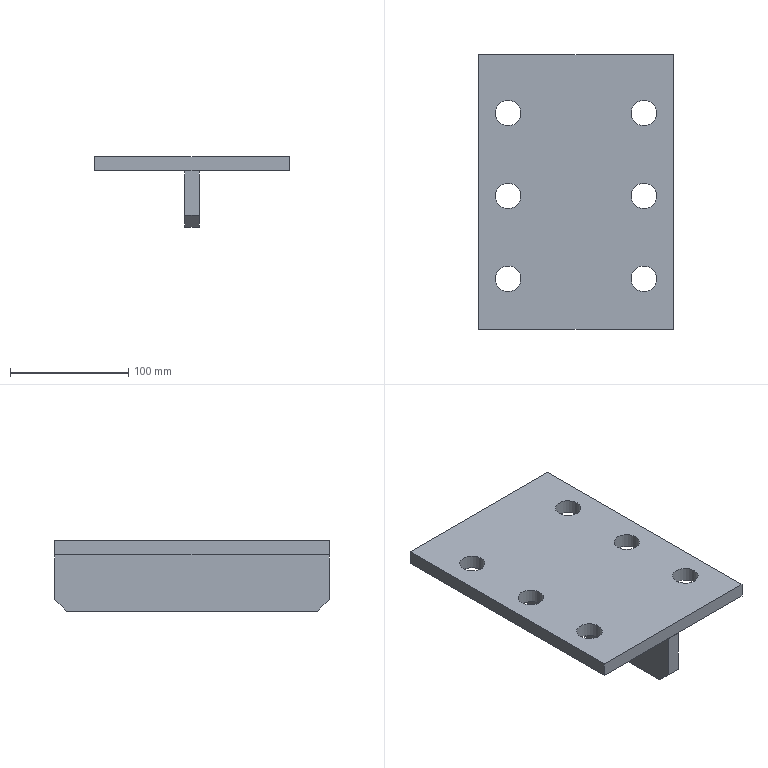Part | STEP file | PN_0033 beam connector 12t_Default<As Machined> | 2 solids | 20 faces | box 164.5 x 232 x 59.5 mm | volume 562868 mm3 | plane 14 | cylinder 6 | commonest cylinder face diameters 21.5 x6
STEP:
#1=CARTESIAN_POINT('',(0.,0.,0.));
#2=DIRECTION('',(0.,0.,1.));
#3=DIRECTION('',(1.,0.,0.));
#4=AXIS2_PLACEMENT_3D('',#1,#2,#3);
#5=CARTESIAN_POINT('',(-6.,-116.,-37.5));
#6=VERTEX_POINT('',#5);
#7=CARTESIAN_POINT('',(6.,-116.,-37.5));
#8=VERTEX_POINT('',#7);
#9=CARTESIAN_POINT('',(6.,-116.,-37.5));
#10=DIRECTION('',(1.,0.,0.));
#11=VECTOR('',#10,1.);
#12=LINE('',#9,#11);
#13=CARTESIAN_POINT('',(6.,-116.,-37.5));
#14=DIRECTION('',(0.,0.7071,0.7071));
#15=DIRECTION('',(1.,0.,0.));
#16=AXIS2_PLACEMENT_3D('',#13,#14,#15);
#17=PLANE('',#16);
#18=CARTESIAN_POINT('',(0.,0.));
#19=DIRECTION('',(1.,0.));
#20=VECTOR('',#19,1.);
#21=LINE('',#18,#20);
#22=(GEOMETRIC_REPRESENTATION_CONTEXT(2)PARAMETRIC_REPRESENTATION_CONTEXT()REPRESENTATION_CONTEXT('',''));
#23=DEFINITIONAL_REPRESENTATION('',(#21),#22);
#24=PCURVE('',#17,#23);
#25=CARTESIAN_POINT('',(6.,-116.,0.));
#26=DIRECTION('',(0.,1.,0.));
#27=DIRECTION('',(0.,0.,1.));
#28=AXIS2_PLACEMENT_3D('',#25,#26,#27);
#29=PLANE('',#28);
#30=CARTESIAN_POINT('',(-37.5,0.));
#31=DIRECTION('',(0.,1.));
#32=VECTOR('',#31,1.);
#33=LINE('',#30,#32);
#34=(GEOMETRIC_REPRESENTATION_CONTEXT(2)PARAMETRIC_REPRESENTATION_CONTEXT()REPRESENTATION_CONTEXT('',''));
#35=DEFINITIONAL_REPRESENTATION('',(#33),#34);
#36=PCURVE('',#29,#35);
#37=SURFACE_CURVE('',#12,(#24,#36),.PCURVE_S1.);
#38=EDGE_CURVE('',#6,#8,#37,.T.);
#39=ORIENTED_EDGE('',*,*,#38,.F.);
#40=CARTESIAN_POINT('',(-6.,-106.,-47.5));
#41=VERTEX_POINT('',#40);
#42=CARTESIAN_POINT('',(-6.,-116.,-37.5));
#43=DIRECTION('',(0.,-0.7071,0.7071));
#44=VECTOR('',#43,1.);
#45=LINE('',#42,#44);
#46=CARTESIAN_POINT('',(-12.,0.));
#47=DIRECTION('',(0.,-1.));
#48=VECTOR('',#47,1.);
#49=LINE('',#46,#48);
#50=(GEOMETRIC_REPRESENTATION_CONTEXT(2)PARAMETRIC_REPRESENTATION_CONTEXT()REPRESENTATION_CONTEXT('',''));
#51=DEFINITIONAL_REPRESENTATION('',(#49),#50);
#52=PCURVE('',#17,#51);
#53=CARTESIAN_POINT('',(-6.,0.,-23.75));
#54=DIRECTION('',(1.,0.,0.));
#55=DIRECTION('',(0.,0.,-1.));
#56=AXIS2_PLACEMENT_3D('',#53,#54,#55);
#57=PLANE('',#56);
#58=CARTESIAN_POINT('',(13.75,-116.));
#59=DIRECTION('',(-0.7071,-0.7071));
#60=VECTOR('',#59,1.);
#61=LINE('',#58,#60);
#62=(GEOMETRIC_REPRESENTATION_CONTEXT(2)PARAMETRIC_REPRESENTATION_CONTEXT()REPRESENTATION_CONTEXT('',''));
#63=DEFINITIONAL_REPRESENTATION('',(#61),#62);
#64=PCURVE('',#57,#63);
#65=SURFACE_CURVE('',#45,(#52,#64),.PCURVE_S1.);
#66=EDGE_CURVE('',#41,#6,#65,.T.);
#67=ORIENTED_EDGE('',*,*,#66,.F.);
#68=CARTESIAN_POINT('',(6.,-106.,-47.5));
#69=VERTEX_POINT('',#68);
#70=CARTESIAN_POINT('',(6.,-106.,-47.5));
#71=DIRECTION('',(-1.,0.,0.));
#72=VECTOR('',#71,1.);
#73=LINE('',#70,#72);
#74=CARTESIAN_POINT('',(0.,14.142));
#75=DIRECTION('',(-1.,0.));
#76=VECTOR('',#75,1.);
#77=LINE('',#74,#76);
#78=(GEOMETRIC_REPRESENTATION_CONTEXT(2)PARAMETRIC_REPRESENTATION_CONTEXT()REPRESENTATION_CONTEXT('',''));
#79=DEFINITIONAL_REPRESENTATION('',(#77),#78);
#80=PCURVE('',#17,#79);
#81=CARTESIAN_POINT('',(6.,116.,-47.5));
#82=DIRECTION('',(0.,0.,1.));
#83=DIRECTION('',(1.,0.,0.));
#84=AXIS2_PLACEMENT_3D('',#81,#82,#83);
#85=PLANE('',#84);
#86=CARTESIAN_POINT('',(0.,-222.));
#87=DIRECTION('',(-1.,0.));
#88=VECTOR('',#87,1.);
#89=LINE('',#86,#88);
#90=(GEOMETRIC_REPRESENTATION_CONTEXT(2)PARAMETRIC_REPRESENTATION_CONTEXT()REPRESENTATION_CONTEXT('',''));
#91=DEFINITIONAL_REPRESENTATION('',(#89),#90);
#92=PCURVE('',#85,#91);
#93=SURFACE_CURVE('',#73,(#80,#92),.PCURVE_S1.);
#94=EDGE_CURVE('',#69,#41,#93,.T.);
#95=ORIENTED_EDGE('',*,*,#94,.F.);
#96=CARTESIAN_POINT('',(6.,-64.875,-88.625));
#97=DIRECTION('',(0.,0.7071,-0.7071));
#98=VECTOR('',#97,1.);
#99=LINE('',#96,#98);
#100=CARTESIAN_POINT('',(0.,72.302));
#101=DIRECTION('',(0.,1.));
#102=VECTOR('',#101,1.);
#103=LINE('',#100,#102);
#104=(GEOMETRIC_REPRESENTATION_CONTEXT(2)PARAMETRIC_REPRESENTATION_CONTEXT()REPRESENTATION_CONTEXT('',''));
#105=DEFINITIONAL_REPRESENTATION('',(#103),#104);
#106=PCURVE('',#17,#105);
#107=CARTESIAN_POINT('',(6.,0.,-23.75));
#108=DIRECTION('',(1.,0.,0.));
#109=DIRECTION('',(0.,0.,-1.));
#110=AXIS2_PLACEMENT_3D('',#107,#108,#109);
#111=PLANE('',#110);
#112=CARTESIAN_POINT('',(64.875,-64.875));
#113=DIRECTION('',(0.7071,0.7071));
#114=VECTOR('',#113,1.);
#115=LINE('',#112,#114);
#116=(GEOMETRIC_REPRESENTATION_CONTEXT(2)PARAMETRIC_REPRESENTATION_CONTEXT()REPRESENTATION_CONTEXT('',''));
#117=DEFINITIONAL_REPRESENTATION('',(#115),#116);
#118=PCURVE('',#111,#117);
#119=SURFACE_CURVE('',#99,(#106,#118),.PCURVE_S1.);
#120=EDGE_CURVE('',#8,#69,#119,.T.);
#121=ORIENTED_EDGE('',*,*,#120,.F.);
#122=EDGE_LOOP('',(#39,#67,#95,#121));
#123=FACE_BOUND('',#122,.T.);
#124=ADVANCED_FACE('',(#123),#17,.F.);
#125=CARTESIAN_POINT('',(6.,116.,-37.5));
#126=VERTEX_POINT('',#125);
#127=CARTESIAN_POINT('',(-6.,116.,-37.5));
#128=VERTEX_POINT('',#127);
#129=CARTESIAN_POINT('',(6.,116.,-37.5));
#130=DIRECTION('',(-1.,0.,0.));
#131=VECTOR('',#130,1.);
#132=LINE('',#129,#131);
#133=CARTESIAN_POINT('',(6.,116.,-37.5));
#134=DIRECTION('',(0.,-0.7071,0.7071));
#135=DIRECTION('',(-1.,0.,0.));
#136=AXIS2_PLACEMENT_3D('',#133,#134,#135);
#137=PLANE('',#136);
#138=CARTESIAN_POINT('',(0.,0.));
#139=DIRECTION('',(1.,0.));
#140=VECTOR('',#139,1.);
#141=LINE('',#138,#140);
#142=(GEOMETRIC_REPRESENTATION_CONTEXT(2)PARAMETRIC_REPRESENTATION_CONTEXT()REPRESENTATION_CONTEXT('',''));
#143=DEFINITIONAL_REPRESENTATION('',(#141),#142);
#144=PCURVE('',#137,#143);
#145=CARTESIAN_POINT('',(6.,116.,0.));
#146=DIRECTION('',(0.,-1.,0.));
#147=DIRECTION('',(0.,0.,-1.));
#148=AXIS2_PLACEMENT_3D('',#145,#146,#147);
#149=PLANE('',#148);
#150=CARTESIAN_POINT('',(37.5,0.));
#151=DIRECTION('',(0.,-1.));
#152=VECTOR('',#151,1.);
#153=LINE('',#150,#152);
#154=(GEOMETRIC_REPRESENTATION_CONTEXT(2)PARAMETRIC_REPRESENTATION_CONTEXT()REPRESENTATION_CONTEXT('',''));
#155=DEFINITIONAL_REPRESENTATION('',(#153),#154);
#156=PCURVE('',#149,#155);
#157=SURFACE_CURVE('',#132,(#144,#156),.PCURVE_S1.);
#158=EDGE_CURVE('',#126,#128,#157,.T.);
#159=ORIENTED_EDGE('',*,*,#158,.F.);
#160=CARTESIAN_POINT('',(6.,106.,-47.5));
#161=VERTEX_POINT('',#160);
#162=CARTESIAN_POINT('',(6.,64.875,-88.625));
#163=DIRECTION('',(0.,0.7071,0.7071));
#164=VECTOR('',#163,1.);
#165=LINE('',#162,#164);
#166=CARTESIAN_POINT('',(0.,72.302));
#167=DIRECTION('',(0.,-1.));
#168=VECTOR('',#167,1.);
#169=LINE('',#166,#168);
#170=(GEOMETRIC_REPRESENTATION_CONTEXT(2)PARAMETRIC_REPRESENTATION_CONTEXT()REPRESENTATION_CONTEXT('',''));
#171=DEFINITIONAL_REPRESENTATION('',(#169),#170);
#172=PCURVE('',#137,#171);
#173=CARTESIAN_POINT('',(64.875,64.875));
#174=DIRECTION('',(-0.7071,0.7071));
#175=VECTOR('',#174,1.);
#176=LINE('',#173,#175);
#177=(GEOMETRIC_REPRESENTATION_CONTEXT(2)PARAMETRIC_REPRESENTATION_CONTEXT()REPRESENTATION_CONTEXT('',''));
#178=DEFINITIONAL_REPRESENTATION('',(#176),#177);
#179=PCURVE('',#111,#178);
#180=SURFACE_CURVE('',#165,(#172,#179),.PCURVE_S1.);
#181=EDGE_CURVE('',#161,#126,#180,.T.);
#182=ORIENTED_EDGE('',*,*,#181,.F.);
#183=CARTESIAN_POINT('',(-6.,106.,-47.5));
#184=VERTEX_POINT('',#183);
#185=CARTESIAN_POINT('',(6.,106.,-47.5));
#186=DIRECTION('',(1.,0.,0.));
#187=VECTOR('',#186,1.);
#188=LINE('',#185,#187);
#189=CARTESIAN_POINT('',(0.,14.142));
#190=DIRECTION('',(-1.,0.));
#191=VECTOR('',#190,1.);
#192=LINE('',#189,#191);
#193=(GEOMETRIC_REPRESENTATION_CONTEXT(2)PARAMETRIC_REPRESENTATION_CONTEXT()REPRESENTATION_CONTEXT('',''));
#194=DEFINITIONAL_REPRESENTATION('',(#192),#193);
#195=PCURVE('',#137,#194);
#196=CARTESIAN_POINT('',(0.,-10.));
#197=DIRECTION('',(1.,0.));
#198=VECTOR('',#197,1.);
#199=LINE('',#196,#198);
#200=(GEOMETRIC_REPRESENTATION_CONTEXT(2)PARAMETRIC_REPRESENTATION_CONTEXT()REPRESENTATION_CONTEXT('',''));
#201=DEFINITIONAL_REPRESENTATION('',(#199),#200);
#202=PCURVE('',#85,#201);
#203=SURFACE_CURVE('',#188,(#195,#202),.PCURVE_S1.);
#204=EDGE_CURVE('',#184,#161,#203,.T.);
#205=ORIENTED_EDGE('',*,*,#204,.F.);
#206=CARTESIAN_POINT('',(-6.,116.,-37.5));
#207=DIRECTION('',(0.,-0.7071,-0.7071));
#208=VECTOR('',#207,1.);
#209=LINE('',#206,#208);
#210=CARTESIAN_POINT('',(12.,0.));
#211=DIRECTION('',(0.,1.));
#212=VECTOR('',#211,1.);
#213=LINE('',#210,#212);
#214=(GEOMETRIC_REPRESENTATION_CONTEXT(2)PARAMETRIC_REPRESENTATION_CONTEXT()REPRESENTATION_CONTEXT('',''));
#215=DEFINITIONAL_REPRESENTATION('',(#213),#214);
#216=PCURVE('',#137,#215);
#217=CARTESIAN_POINT('',(13.75,116.));
#218=DIRECTION('',(0.7071,-0.7071));
#219=VECTOR('',#218,1.);
#220=LINE('',#217,#219);
#221=(GEOMETRIC_REPRESENTATION_CONTEXT(2)PARAMETRIC_REPRESENTATION_CONTEXT()REPRESENTATION_CONTEXT('',''));
#222=DEFINITIONAL_REPRESENTATION('',(#220),#221);
#223=PCURVE('',#57,#222);
#224=SURFACE_CURVE('',#209,(#216,#223),.PCURVE_S1.);
#225=EDGE_CURVE('',#128,#184,#224,.T.);
#226=ORIENTED_EDGE('',*,*,#225,.F.);
#227=EDGE_LOOP('',(#159,#182,#205,#226));
#228=FACE_BOUND('',#227,.T.);
#229=ADVANCED_FACE('',(#228),#137,.F.);
#230=CARTESIAN_POINT('',(6.,116.,-47.5));
#231=DIRECTION('',(0.,1.,0.));
#232=VECTOR('',#231,1.);
#233=LINE('',#230,#232);
#234=CARTESIAN_POINT('',(0.,0.));
#235=DIRECTION('',(0.,1.));
#236=VECTOR('',#235,1.);
#237=LINE('',#234,#236);
#238=(GEOMETRIC_REPRESENTATION_CONTEXT(2)PARAMETRIC_REPRESENTATION_CONTEXT()REPRESENTATION_CONTEXT('',''));
#239=DEFINITIONAL_REPRESENTATION('',(#237),#238);
#240=PCURVE('',#85,#239);
#241=CARTESIAN_POINT('',(23.75,116.));
#242=DIRECTION('',(0.,1.));
#243=VECTOR('',#242,1.);
#244=LINE('',#241,#243);
#245=(GEOMETRIC_REPRESENTATION_CONTEXT(2)PARAMETRIC_REPRESENTATION_CONTEXT()REPRESENTATION_CONTEXT('',''));
#246=DEFINITIONAL_REPRESENTATION('',(#244),#245);
#247=PCURVE('',#111,#246);
#248=SURFACE_CURVE('',#233,(#240,#247),.PCURVE_S1.);
#249=EDGE_CURVE('',#69,#161,#248,.T.);
#250=ORIENTED_EDGE('',*,*,#249,.F.);
#251=ORIENTED_EDGE('',*,*,#94,.T.);
#252=CARTESIAN_POINT('',(-6.,116.,-47.5));
#253=DIRECTION('',(0.,1.,0.));
#254=VECTOR('',#253,1.);
#255=LINE('',#252,#254);
#256=CARTESIAN_POINT('',(-12.,0.));
#257=DIRECTION('',(0.,1.));
#258=VECTOR('',#257,1.);
#259=LINE('',#256,#258);
#260=(GEOMETRIC_REPRESENTATION_CONTEXT(2)PARAMETRIC_REPRESENTATION_CONTEXT()REPRESENTATION_CONTEXT('',''));
#261=DEFINITIONAL_REPRESENTATION('',(#259),#260);
#262=PCURVE('',#85,#261);
#263=CARTESIAN_POINT('',(23.75,116.));
#264=DIRECTION('',(0.,1.));
#265=VECTOR('',#264,1.);
#266=LINE('',#263,#265);
#267=(GEOMETRIC_REPRESENTATION_CONTEXT(2)PARAMETRIC_REPRESENTATION_CONTEXT()REPRESENTATION_CONTEXT('',''));
#268=DEFINITIONAL_REPRESENTATION('',(#266),#267);
#269=PCURVE('',#57,#268);
#270=SURFACE_CURVE('',#255,(#262,#269),.PCURVE_S1.);
#271=EDGE_CURVE('',#41,#184,#270,.T.);
#272=ORIENTED_EDGE('',*,*,#271,.T.);
#273=ORIENTED_EDGE('',*,*,#204,.T.);
#274=EDGE_LOOP('',(#250,#251,#272,#273));
#275=FACE_BOUND('',#274,.T.);
#276=ADVANCED_FACE('',(#275),#85,.F.);
#277=CARTESIAN_POINT('',(6.,116.,0.));
#278=VERTEX_POINT('',#277);
#279=CARTESIAN_POINT('',(6.,116.,0.));
#280=DIRECTION('',(0.,0.,1.));
#281=VECTOR('',#280,1.);
#282=LINE('',#279,#281);
#283=CARTESIAN_POINT('',(0.,0.));
#284=DIRECTION('',(-1.,0.));
#285=VECTOR('',#284,1.);
#286=LINE('',#283,#285);
#287=(GEOMETRIC_REPRESENTATION_CONTEXT(2)PARAMETRIC_REPRESENTATION_CONTEXT()REPRESENTATION_CONTEXT('',''));
#288=DEFINITIONAL_REPRESENTATION('',(#286),#287);
#289=PCURVE('',#149,#288);
#290=CARTESIAN_POINT('',(-23.75,116.));
#291=DIRECTION('',(-1.,0.));
#292=VECTOR('',#291,1.);
#293=LINE('',#290,#292);
#294=(GEOMETRIC_REPRESENTATION_CONTEXT(2)PARAMETRIC_REPRESENTATION_CONTEXT()REPRESENTATION_CONTEXT('',''));
#295=DEFINITIONAL_REPRESENTATION('',(#293),#294);
#296=PCURVE('',#111,#295);
#297=SURFACE_CURVE('',#282,(#289,#296),.PCURVE_S1.);
#298=EDGE_CURVE('',#126,#278,#297,.T.);
#299=ORIENTED_EDGE('',*,*,#298,.F.);
#300=ORIENTED_EDGE('',*,*,#158,.T.);
#301=CARTESIAN_POINT('',(-6.,116.,0.));
#302=VERTEX_POINT('',#301);
#303=CARTESIAN_POINT('',(-6.,116.,0.));
#304=DIRECTION('',(0.,0.,1.));
#305=VECTOR('',#304,1.);
#306=LINE('',#303,#305);
#307=CARTESIAN_POINT('',(0.,-12.));
#308=DIRECTION('',(-1.,0.));
#309=VECTOR('',#308,1.);
#310=LINE('',#307,#309);
#311=(GEOMETRIC_REPRESENTATION_CONTEXT(2)PARAMETRIC_REPRESENTATION_CONTEXT()REPRESENTATION_CONTEXT('',''));
#312=DEFINITIONAL_REPRESENTATION('',(#310),#311);
#313=PCURVE('',#149,#312);
#314=CARTESIAN_POINT('',(-23.75,116.));
#315=DIRECTION('',(-1.,0.));
#316=VECTOR('',#315,1.);
#317=LINE('',#314,#316);
#318=(GEOMETRIC_REPRESENTATION_CONTEXT(2)PARAMETRIC_REPRESENTATION_CONTEXT()REPRESENTATION_CONTEXT('',''));
#319=DEFINITIONAL_REPRESENTATION('',(#317),#318);
#320=PCURVE('',#57,#319);
#321=SURFACE_CURVE('',#306,(#313,#320),.PCURVE_S1.);
#322=EDGE_CURVE('',#128,#302,#321,.T.);
#323=ORIENTED_EDGE('',*,*,#322,.T.);
#324=CARTESIAN_POINT('',(6.,116.,0.));
#325=DIRECTION('',(-1.,0.,0.));
#326=VECTOR('',#325,1.);
#327=LINE('',#324,#326);
#328=CARTESIAN_POINT('',(0.,0.));
#329=DIRECTION('',(0.,-1.));
#330=VECTOR('',#329,1.);
#331=LINE('',#328,#330);
#332=(GEOMETRIC_REPRESENTATION_CONTEXT(2)PARAMETRIC_REPRESENTATION_CONTEXT()REPRESENTATION_CONTEXT('',''));
#333=DEFINITIONAL_REPRESENTATION('',(#331),#332);
#334=PCURVE('',#149,#333);
#335=CARTESIAN_POINT('',(6.,116.,0.));
#336=DIRECTION('',(0.,0.,-1.));
#337=DIRECTION('',(-1.,0.,0.));
#338=AXIS2_PLACEMENT_3D('',#335,#336,#337);
#339=PLANE('',#338);
#340=CARTESIAN_POINT('',(0.,0.));
#341=DIRECTION('',(1.,0.));
#342=VECTOR('',#341,1.);
#343=LINE('',#340,#342);
#344=(GEOMETRIC_REPRESENTATION_CONTEXT(2)PARAMETRIC_REPRESENTATION_CONTEXT()REPRESENTATION_CONTEXT('',''));
#345=DEFINITIONAL_REPRESENTATION('',(#343),#344);
#346=PCURVE('',#339,#345);
#347=SURFACE_CURVE('',#327,(#334,#346),.PCURVE_S1.);
#348=EDGE_CURVE('',#278,#302,#347,.T.);
#349=ORIENTED_EDGE('',*,*,#348,.F.);
#350=EDGE_LOOP('',(#299,#300,#323,#349));
#351=FACE_BOUND('',#350,.T.);
#352=ADVANCED_FACE('',(#351),#149,.F.);
#353=CARTESIAN_POINT('',(-6.,-116.,0.));
#354=VERTEX_POINT('',#353);
#355=CARTESIAN_POINT('',(-6.,116.,0.));
#356=DIRECTION('',(0.,-1.,0.));
#357=VECTOR('',#356,1.);
#358=LINE('',#355,#357);
#359=CARTESIAN_POINT('',(12.,0.));
#360=DIRECTION('',(0.,-1.));
#361=VECTOR('',#360,1.);
#362=LINE('',#359,#361);
#363=(GEOMETRIC_REPRESENTATION_CONTEXT(2)PARAMETRIC_REPRESENTATION_CONTEXT()REPRESENTATION_CONTEXT('',''));
#364=DEFINITIONAL_REPRESENTATION('',(#362),#363);
#365=PCURVE('',#339,#364);
#366=CARTESIAN_POINT('',(-23.75,116.));
#367=DIRECTION('',(0.,-1.));
#368=VECTOR('',#367,1.);
#369=LINE('',#366,#368);
#370=(GEOMETRIC_REPRESENTATION_CONTEXT(2)PARAMETRIC_REPRESENTATION_CONTEXT()REPRESENTATION_CONTEXT('',''));
#371=DEFINITIONAL_REPRESENTATION('',(#369),#370);
#372=PCURVE('',#57,#371);
#373=SURFACE_CURVE('',#358,(#365,#372),.PCURVE_S1.);
#374=EDGE_CURVE('',#302,#354,#373,.T.);
#375=ORIENTED_EDGE('',*,*,#374,.T.);
#376=CARTESIAN_POINT('',(6.,-116.,0.));
#377=VERTEX_POINT('',#376);
#378=CARTESIAN_POINT('',(6.,-116.,0.));
#379=DIRECTION('',(-1.,0.,0.));
#380=VECTOR('',#379,1.);
#381=LINE('',#378,#380);
#382=CARTESIAN_POINT('',(0.,-232.));
#383=DIRECTION('',(1.,0.));
#384=VECTOR('',#383,1.);
#385=LINE('',#382,#384);
#386=(GEOMETRIC_REPRESENTATION_CONTEXT(2)PARAMETRIC_REPRESENTATION_CONTEXT()REPRESENTATION_CONTEXT('',''));
#387=DEFINITIONAL_REPRESENTATION('',(#385),#386);
#388=PCURVE('',#339,#387);
#389=CARTESIAN_POINT('',(0.,0.));
#390=DIRECTION('',(0.,-1.));
#391=VECTOR('',#390,1.);
#392=LINE('',#389,#391);
#393=(GEOMETRIC_REPRESENTATION_CONTEXT(2)PARAMETRIC_REPRESENTATION_CONTEXT()REPRESENTATION_CONTEXT('',''));
#394=DEFINITIONAL_REPRESENTATION('',(#392),#393);
#395=PCURVE('',#29,#394);
#396=SURFACE_CURVE('',#381,(#388,#395),.PCURVE_S1.);
#397=EDGE_CURVE('',#377,#354,#396,.T.);
#398=ORIENTED_EDGE('',*,*,#397,.F.);
#399=CARTESIAN_POINT('',(6.,116.,0.));
#400=DIRECTION('',(0.,-1.,0.));
#401=VECTOR('',#400,1.);
#402=LINE('',#399,#401);
#403=CARTESIAN_POINT('',(0.,0.));
#404=DIRECTION('',(0.,-1.));
#405=VECTOR('',#404,1.);
#406=LINE('',#403,#405);
#407=(GEOMETRIC_REPRESENTATION_CONTEXT(2)PARAMETRIC_REPRESENTATION_CONTEXT()REPRESENTATION_CONTEXT('',''));
#408=DEFINITIONAL_REPRESENTATION('',(#406),#407);
#409=PCURVE('',#339,#408);
#410=CARTESIAN_POINT('',(-23.75,116.));
#411=DIRECTION('',(0.,-1.));
#412=VECTOR('',#411,1.);
#413=LINE('',#410,#412);
#414=(GEOMETRIC_REPRESENTATION_CONTEXT(2)PARAMETRIC_REPRESENTATION_CONTEXT()REPRESENTATION_CONTEXT('',''));
#415=DEFINITIONAL_REPRESENTATION('',(#413),#414);
#416=PCURVE('',#111,#415);
#417=SURFACE_CURVE('',#402,(#409,#416),.PCURVE_S1.);
#418=EDGE_CURVE('',#278,#377,#417,.T.);
#419=ORIENTED_EDGE('',*,*,#418,.F.);
#420=ORIENTED_EDGE('',*,*,#348,.T.);
#421=EDGE_LOOP('',(#375,#398,#419,#420));
#422=FACE_BOUND('',#421,.T.);
#423=ADVANCED_FACE('',(#422),#339,.F.);
#424=CARTESIAN_POINT('',(-6.,-116.,0.));
#425=DIRECTION('',(0.,0.,-1.));
#426=VECTOR('',#425,1.);
#427=LINE('',#424,#426);
#428=CARTESIAN_POINT('',(0.,-12.));
#429=DIRECTION('',(-1.,0.));
#430=VECTOR('',#429,1.);
#431=LINE('',#428,#430);
#432=(GEOMETRIC_REPRESENTATION_CONTEXT(2)PARAMETRIC_REPRESENTATION_CONTEXT()REPRESENTATION_CONTEXT('',''));
#433=DEFINITIONAL_REPRESENTATION('',(#431),#432);
#434=PCURVE('',#29,#433);
#435=CARTESIAN_POINT('',(-23.75,-116.));
#436=DIRECTION('',(1.,0.));
#437=VECTOR('',#436,1.);
#438=LINE('',#435,#437);
#439=(GEOMETRIC_REPRESENTATION_CONTEXT(2)PARAMETRIC_REPRESENTATION_CONTEXT()REPRESENTATION_CONTEXT('',''));
#440=DEFINITIONAL_REPRESENTATION('',(#438),#439);
#441=PCURVE('',#57,#440);
#442=SURFACE_CURVE('',#427,(#434,#441),.PCURVE_S1.);
#443=EDGE_CURVE('',#354,#6,#442,.T.);
#444=ORIENTED_EDGE('',*,*,#443,.T.);
#445=ORIENTED_EDGE('',*,*,#38,.T.);
#446=CARTESIAN_POINT('',(6.,-116.,0.));
#447=DIRECTION('',(0.,0.,-1.));
#448=VECTOR('',#447,1.);
#449=LINE('',#446,#448);
#450=CARTESIAN_POINT('',(0.,0.));
#451=DIRECTION('',(-1.,0.));
#452=VECTOR('',#451,1.);
#453=LINE('',#450,#452);
#454=(GEOMETRIC_REPRESENTATION_CONTEXT(2)PARAMETRIC_REPRESENTATION_CONTEXT()REPRESENTATION_CONTEXT('',''));
#455=DEFINITIONAL_REPRESENTATION('',(#453),#454);
#456=PCURVE('',#29,#455);
#457=CARTESIAN_POINT('',(-23.75,-116.));
#458=DIRECTION('',(1.,0.));
#459=VECTOR('',#458,1.);
#460=LINE('',#457,#459);
#461=(GEOMETRIC_REPRESENTATION_CONTEXT(2)PARAMETRIC_REPRESENTATION_CONTEXT()REPRESENTATION_CONTEXT('',''));
#462=DEFINITIONAL_REPRESENTATION('',(#460),#461);
#463=PCURVE('',#111,#462);
#464=SURFACE_CURVE('',#449,(#456,#463),.PCURVE_S1.);
#465=EDGE_CURVE('',#377,#8,#464,.T.);
#466=ORIENTED_EDGE('',*,*,#465,.F.);
#467=ORIENTED_EDGE('',*,*,#397,.T.);
#468=EDGE_LOOP('',(#444,#445,#466,#467));
#469=FACE_BOUND('',#468,.T.);
#470=ADVANCED_FACE('',(#469),#29,.F.);
#471=ORIENTED_EDGE('',*,*,#465,.T.);
#472=ORIENTED_EDGE('',*,*,#120,.T.);
#473=ORIENTED_EDGE('',*,*,#249,.T.);
#474=ORIENTED_EDGE('',*,*,#181,.T.);
#475=ORIENTED_EDGE('',*,*,#298,.T.);
#476=ORIENTED_EDGE('',*,*,#418,.T.);
#477=EDGE_LOOP('',(#471,#472,#473,#474,#475,#476));
#478=FACE_BOUND('',#477,.T.);
#479=ADVANCED_FACE('',(#478),#111,.T.);
#480=ORIENTED_EDGE('',*,*,#271,.F.);
#481=ORIENTED_EDGE('',*,*,#66,.T.);
#482=ORIENTED_EDGE('',*,*,#443,.F.);
#483=ORIENTED_EDGE('',*,*,#374,.F.);
#484=ORIENTED_EDGE('',*,*,#322,.F.);
#485=ORIENTED_EDGE('',*,*,#225,.T.);
#486=EDGE_LOOP('',(#480,#481,#482,#483,#484,#485));
#487=FACE_BOUND('',#486,.T.);
#488=ADVANCED_FACE('',(#487),#57,.F.);
#489=CLOSED_SHELL('',(#124,#229,#276,#352,#423,#470,#479,#488));
#490=MANIFOLD_SOLID_BREP('',#489);
#491=CARTESIAN_POINT('',(82.25,-116.,0.));
#492=VERTEX_POINT('',#491);
#493=CARTESIAN_POINT('',(82.25,116.,0.));
#494=VERTEX_POINT('',#493);
#495=CARTESIAN_POINT('',(82.25,116.,0.));
#496=DIRECTION('',(0.,1.,0.));
#497=VECTOR('',#496,1.);
#498=LINE('',#495,#497);
#499=CARTESIAN_POINT('',(82.25,116.,12.));
#500=DIRECTION('',(-1.,0.,0.));
#501=DIRECTION('',(0.,0.,1.));
#502=AXIS2_PLACEMENT_3D('',#499,#500,#501);
#503=PLANE('',#502);
#504=CARTESIAN_POINT('',(-12.,0.));
#505=DIRECTION('',(0.,1.));
#506=VECTOR('',#505,1.);
#507=LINE('',#504,#506);
#508=(GEOMETRIC_REPRESENTATION_CONTEXT(2)PARAMETRIC_REPRESENTATION_CONTEXT()REPRESENTATION_CONTEXT('',''));
#509=DEFINITIONAL_REPRESENTATION('',(#507),#508);
#510=PCURVE('',#503,#509);
#511=CARTESIAN_POINT('',(0.,0.,0.));
#512=DIRECTION('',(0.,0.,1.));
#513=DIRECTION('',(1.,0.,0.));
#514=AXIS2_PLACEMENT_3D('',#511,#512,#513);
#515=PLANE('',#514);
#516=CARTESIAN_POINT('',(82.25,116.));
#517=DIRECTION('',(0.,1.));
#518=VECTOR('',#517,1.);
#519=LINE('',#516,#518);
#520=(GEOMETRIC_REPRESENTATION_CONTEXT(2)PARAMETRIC_REPRESENTATION_CONTEXT()REPRESENTATION_CONTEXT('',''));
#521=DEFINITIONAL_REPRESENTATION('',(#519),#520);
#522=PCURVE('',#515,#521);
#523=SURFACE_CURVE('',#498,(#510,#522),.PCURVE_S1.);
#524=EDGE_CURVE('',#492,#494,#523,.T.);
#525=ORIENTED_EDGE('',*,*,#524,.T.);
#526=CARTESIAN_POINT('',(82.25,116.,12.));
#527=VERTEX_POINT('',#526);
#528=CARTESIAN_POINT('',(82.25,116.,12.));
#529=DIRECTION('',(0.,0.,-1.));
#530=VECTOR('',#529,1.);
#531=LINE('',#528,#530);
#532=CARTESIAN_POINT('',(0.,0.));
#533=DIRECTION('',(-1.,0.));
#534=VECTOR('',#533,1.);
#535=LINE('',#532,#534);
#536=(GEOMETRIC_REPRESENTATION_CONTEXT(2)PARAMETRIC_REPRESENTATION_CONTEXT()REPRESENTATION_CONTEXT('',''));
#537=DEFINITIONAL_REPRESENTATION('',(#535),#536);
#538=PCURVE('',#503,#537);
#539=CARTESIAN_POINT('',(-82.25,116.,12.));
#540=DIRECTION('',(0.,-1.,0.));
#541=DIRECTION('',(0.,0.,-1.));
#542=AXIS2_PLACEMENT_3D('',#539,#540,#541);
#543=PLANE('',#542);
#544=CARTESIAN_POINT('',(0.,164.5));
#545=DIRECTION('',(1.,0.));
#546=VECTOR('',#545,1.);
#547=LINE('',#544,#546);
#548=(GEOMETRIC_REPRESENTATION_CONTEXT(2)PARAMETRIC_REPRESENTATION_CONTEXT()REPRESENTATION_CONTEXT('',''));
#549=DEFINITIONAL_REPRESENTATION('',(#547),#548);
#550=PCURVE('',#543,#549);
#551=SURFACE_CURVE('',#531,(#538,#550),.PCURVE_S1.);
#552=EDGE_CURVE('',#527,#494,#551,.T.);
#553=ORIENTED_EDGE('',*,*,#552,.F.);
#554=CARTESIAN_POINT('',(82.25,-116.,12.));
#555=VERTEX_POINT('',#554);
#556=CARTESIAN_POINT('',(82.25,116.,12.));
#557=DIRECTION('',(0.,1.,0.));
#558=VECTOR('',#557,1.);
#559=LINE('',#556,#558);
#560=CARTESIAN_POINT('',(0.,0.));
#561=DIRECTION('',(0.,1.));
#562=VECTOR('',#561,1.);
#563=LINE('',#560,#562);
#564=(GEOMETRIC_REPRESENTATION_CONTEXT(2)PARAMETRIC_REPRESENTATION_CONTEXT()REPRESENTATION_CONTEXT('',''));
#565=DEFINITIONAL_REPRESENTATION('',(#563),#564);
#566=PCURVE('',#503,#565);
#567=CARTESIAN_POINT('',(0.,0.,12.));
#568=DIRECTION('',(0.,0.,1.));
#569=DIRECTION('',(1.,0.,0.));
#570=AXIS2_PLACEMENT_3D('',#567,#568,#569);
#571=PLANE('',#570);
#572=CARTESIAN_POINT('',(82.25,116.));
#573=DIRECTION('',(0.,1.));
#574=VECTOR('',#573,1.);
#575=LINE('',#572,#574);
#576=(GEOMETRIC_REPRESENTATION_CONTEXT(2)PARAMETRIC_REPRESENTATION_CONTEXT()REPRESENTATION_CONTEXT('',''));
#577=DEFINITIONAL_REPRESENTATION('',(#575),#576);
#578=PCURVE('',#571,#577);
#579=SURFACE_CURVE('',#559,(#566,#578),.PCURVE_S1.);
#580=EDGE_CURVE('',#555,#527,#579,.T.);
#581=ORIENTED_EDGE('',*,*,#580,.F.);
#582=CARTESIAN_POINT('',(82.25,-116.,12.));
#583=DIRECTION('',(0.,0.,-1.));
#584=VECTOR('',#583,1.);
#585=LINE('',#582,#584);
#586=CARTESIAN_POINT('',(0.,-232.));
#587=DIRECTION('',(-1.,0.));
#588=VECTOR('',#587,1.);
#589=LINE('',#586,#588);
#590=(GEOMETRIC_REPRESENTATION_CONTEXT(2)PARAMETRIC_REPRESENTATION_CONTEXT()REPRESENTATION_CONTEXT('',''));
#591=DEFINITIONAL_REPRESENTATION('',(#589),#590);
#592=PCURVE('',#503,#591);
#593=CARTESIAN_POINT('',(-82.25,-116.,12.));
#594=DIRECTION('',(0.,1.,0.));
#595=DIRECTION('',(0.,0.,1.));
#596=AXIS2_PLACEMENT_3D('',#593,#594,#595);
#597=PLANE('',#596);
#598=CARTESIAN_POINT('',(0.,164.5));
#599=DIRECTION('',(-1.,0.));
#600=VECTOR('',#599,1.);
#601=LINE('',#598,#600);
#602=(GEOMETRIC_REPRESENTATION_CONTEXT(2)PARAMETRIC_REPRESENTATION_CONTEXT()REPRESENTATION_CONTEXT('',''));
#603=DEFINITIONAL_REPRESENTATION('',(#601),#602);
#604=PCURVE('',#597,#603);
#605=SURFACE_CURVE('',#585,(#592,#604),.PCURVE_S1.);
#606=EDGE_CURVE('',#555,#492,#605,.T.);
#607=ORIENTED_EDGE('',*,*,#606,.T.);
#608=EDGE_LOOP('',(#525,#553,#581,#607));
#609=FACE_BOUND('',#608,.T.);
#610=ADVANCED_FACE('',(#609),#503,.F.);
#611=CARTESIAN_POINT('',(-82.25,116.,0.));
#612=VERTEX_POINT('',#611);
#613=CARTESIAN_POINT('',(-82.25,116.,0.));
#614=DIRECTION('',(-1.,0.,0.));
#615=VECTOR('',#614,1.);
#616=LINE('',#613,#615);
#617=CARTESIAN_POINT('',(12.,0.));
#618=DIRECTION('',(0.,-1.));
#619=VECTOR('',#618,1.);
#620=LINE('',#617,#619);
#621=(GEOMETRIC_REPRESENTATION_CONTEXT(2)PARAMETRIC_REPRESENTATION_CONTEXT()REPRESENTATION_CONTEXT('',''));
#622=DEFINITIONAL_REPRESENTATION('',(#620),#621);
#623=PCURVE('',#543,#622);
#624=CARTESIAN_POINT('',(-82.25,116.));
#625=DIRECTION('',(-1.,0.));
#626=VECTOR('',#625,1.);
#627=LINE('',#624,#626);
#628=(GEOMETRIC_REPRESENTATION_CONTEXT(2)PARAMETRIC_REPRESENTATION_CONTEXT()REPRESENTATION_CONTEXT('',''));
#629=DEFINITIONAL_REPRESENTATION('',(#627),#628);
#630=PCURVE('',#515,#629);
#631=SURFACE_CURVE('',#616,(#623,#630),.PCURVE_S1.);
#632=EDGE_CURVE('',#494,#612,#631,.T.);
#633=ORIENTED_EDGE('',*,*,#632,.T.);
#634=CARTESIAN_POINT('',(-82.25,116.,12.));
#635=VERTEX_POINT('',#634);
#636=CARTESIAN_POINT('',(-82.25,116.,12.));
#637=DIRECTION('',(0.,0.,-1.));
#638=VECTOR('',#637,1.);
#639=LINE('',#636,#638);
#640=CARTESIAN_POINT('',(0.,0.));
#641=DIRECTION('',(1.,0.));
#642=VECTOR('',#641,1.);
#643=LINE('',#640,#642);
#644=(GEOMETRIC_REPRESENTATION_CONTEXT(2)PARAMETRIC_REPRESENTATION_CONTEXT()REPRESENTATION_CONTEXT('',''));
#645=DEFINITIONAL_REPRESENTATION('',(#643),#644);
#646=PCURVE('',#543,#645);
#647=CARTESIAN_POINT('',(-82.25,116.,12.));
#648=DIRECTION('',(1.,0.,0.));
#649=DIRECTION('',(0.,0.,-1.));
#650=AXIS2_PLACEMENT_3D('',#647,#648,#649);
#651=PLANE('',#650);
#652=CARTESIAN_POINT('',(0.,0.));
#653=DIRECTION('',(1.,0.));
#654=VECTOR('',#653,1.);
#655=LINE('',#652,#654);
#656=(GEOMETRIC_REPRESENTATION_CONTEXT(2)PARAMETRIC_REPRESENTATION_CONTEXT()REPRESENTATION_CONTEXT('',''));
#657=DEFINITIONAL_REPRESENTATION('',(#655),#656);
#658=PCURVE('',#651,#657);
#659=SURFACE_CURVE('',#639,(#646,#658),.PCURVE_S1.);
#660=EDGE_CURVE('',#635,#612,#659,.T.);
#661=ORIENTED_EDGE('',*,*,#660,.F.);
#662=CARTESIAN_POINT('',(-82.25,116.,12.));
#663=DIRECTION('',(-1.,0.,0.));
#664=VECTOR('',#663,1.);
#665=LINE('',#662,#664);
#666=CARTESIAN_POINT('',(0.,0.));
#667=DIRECTION('',(0.,-1.));
#668=VECTOR('',#667,1.);
#669=LINE('',#666,#668);
#670=(GEOMETRIC_REPRESENTATION_CONTEXT(2)PARAMETRIC_REPRESENTATION_CONTEXT()REPRESENTATION_CONTEXT('',''));
#671=DEFINITIONAL_REPRESENTATION('',(#669),#670);
#672=PCURVE('',#543,#671);
#673=CARTESIAN_POINT('',(-82.25,116.));
#674=DIRECTION('',(-1.,0.));
#675=VECTOR('',#674,1.);
#676=LINE('',#673,#675);
#677=(GEOMETRIC_REPRESENTATION_CONTEXT(2)PARAMETRIC_REPRESENTATION_CONTEXT()REPRESENTATION_CONTEXT('',''));
#678=DEFINITIONAL_REPRESENTATION('',(#676),#677);
#679=PCURVE('',#571,#678);
#680=SURFACE_CURVE('',#665,(#672,#679),.PCURVE_S1.);
#681=EDGE_CURVE('',#527,#635,#680,.T.);
#682=ORIENTED_EDGE('',*,*,#681,.F.);
#683=ORIENTED_EDGE('',*,*,#552,.T.);
#684=EDGE_LOOP('',(#633,#661,#682,#683));
#685=FACE_BOUND('',#684,.T.);
#686=ADVANCED_FACE('',(#685),#543,.F.);
#687=CARTESIAN_POINT('',(-82.25,-116.,0.));
#688=VERTEX_POINT('',#687);
#689=CARTESIAN_POINT('',(-82.25,116.,0.));
#690=DIRECTION('',(0.,-1.,0.));
#691=VECTOR('',#690,1.);
#692=LINE('',#689,#691);
#693=CARTESIAN_POINT('',(12.,0.));
#694=DIRECTION('',(0.,-1.));
#695=VECTOR('',#694,1.);
#696=LINE('',#693,#695);
#697=(GEOMETRIC_REPRESENTATION_CONTEXT(2)PARAMETRIC_REPRESENTATION_CONTEXT()REPRESENTATION_CONTEXT('',''));
#698=DEFINITIONAL_REPRESENTATION('',(#696),#697);
#699=PCURVE('',#651,#698);
#700=CARTESIAN_POINT('',(-82.25,116.));
#701=DIRECTION('',(0.,-1.));
#702=VECTOR('',#701,1.);
#703=LINE('',#700,#702);
#704=(GEOMETRIC_REPRESENTATION_CONTEXT(2)PARAMETRIC_REPRESENTATION_CONTEXT()REPRESENTATION_CONTEXT('',''));
#705=DEFINITIONAL_REPRESENTATION('',(#703),#704);
#706=PCURVE('',#515,#705);
#707=SURFACE_CURVE('',#692,(#699,#706),.PCURVE_S1.);
#708=EDGE_CURVE('',#612,#688,#707,.T.);
#709=ORIENTED_EDGE('',*,*,#708,.T.);
#710=CARTESIAN_POINT('',(-82.25,-116.,12.));
#711=VERTEX_POINT('',#710);
#712=CARTESIAN_POINT('',(-82.25,-116.,12.));
#713=DIRECTION('',(0.,0.,-1.));
#714=VECTOR('',#713,1.);
#715=LINE('',#712,#714);
#716=CARTESIAN_POINT('',(0.,-232.));
#717=DIRECTION('',(1.,0.));
#718=VECTOR('',#717,1.);
#719=LINE('',#716,#718);
#720=(GEOMETRIC_REPRESENTATION_CONTEXT(2)PARAMETRIC_REPRESENTATION_CONTEXT()REPRESENTATION_CONTEXT('',''));
#721=DEFINITIONAL_REPRESENTATION('',(#719),#720);
#722=PCURVE('',#651,#721);
#723=CARTESIAN_POINT('',(0.,0.));
#724=DIRECTION('',(-1.,0.));
#725=VECTOR('',#724,1.);
#726=LINE('',#723,#725);
#727=(GEOMETRIC_REPRESENTATION_CONTEXT(2)PARAMETRIC_REPRESENTATION_CONTEXT()REPRESENTATION_CONTEXT('',''));
#728=DEFINITIONAL_REPRESENTATION('',(#726),#727);
#729=PCURVE('',#597,#728);
#730=SURFACE_CURVE('',#715,(#722,#729),.PCURVE_S1.);
#731=EDGE_CURVE('',#711,#688,#730,.T.);
#732=ORIENTED_EDGE('',*,*,#731,.F.);
#733=CARTESIAN_POINT('',(-82.25,116.,12.));
#734=DIRECTION('',(0.,-1.,0.));
#735=VECTOR('',#734,1.);
#736=LINE('',#733,#735);
#737=CARTESIAN_POINT('',(0.,0.));
#738=DIRECTION('',(0.,-1.));
#739=VECTOR('',#738,1.);
#740=LINE('',#737,#739);
#741=(GEOMETRIC_REPRESENTATION_CONTEXT(2)PARAMETRIC_REPRESENTATION_CONTEXT()REPRESENTATION_CONTEXT('',''));
#742=DEFINITIONAL_REPRESENTATION('',(#740),#741);
#743=PCURVE('',#651,#742);
#744=CARTESIAN_POINT('',(-82.25,116.));
#745=DIRECTION('',(0.,-1.));
#746=VECTOR('',#745,1.);
#747=LINE('',#744,#746);
#748=(GEOMETRIC_REPRESENTATION_CONTEXT(2)PARAMETRIC_REPRESENTATION_CONTEXT()REPRESENTATION_CONTEXT('',''));
#749=DEFINITIONAL_REPRESENTATION('',(#747),#748);
#750=PCURVE('',#571,#749);
#751=SURFACE_CURVE('',#736,(#743,#750),.PCURVE_S1.);
#752=EDGE_CURVE('',#635,#711,#751,.T.);
#753=ORIENTED_EDGE('',*,*,#752,.F.);
#754=ORIENTED_EDGE('',*,*,#660,.T.);
#755=EDGE_LOOP('',(#709,#732,#753,#754));
#756=FACE_BOUND('',#755,.T.);
#757=ADVANCED_FACE('',(#756),#651,.F.);
#758=CARTESIAN_POINT('',(-82.25,-116.,0.));
#759=DIRECTION('',(1.,0.,0.));
#760=VECTOR('',#759,1.);
#761=LINE('',#758,#760);
#762=CARTESIAN_POINT('',(-12.,0.));
#763=DIRECTION('',(0.,1.));
#764=VECTOR('',#763,1.);
#765=LINE('',#762,#764);
#766=(GEOMETRIC_REPRESENTATION_CONTEXT(2)PARAMETRIC_REPRESENTATION_CONTEXT()REPRESENTATION_CONTEXT('',''));
#767=DEFINITIONAL_REPRESENTATION('',(#765),#766);
#768=PCURVE('',#597,#767);
#769=CARTESIAN_POINT('',(-82.25,-116.));
#770=DIRECTION('',(1.,0.));
#771=VECTOR('',#770,1.);
#772=LINE('',#769,#771);
#773=(GEOMETRIC_REPRESENTATION_CONTEXT(2)PARAMETRIC_REPRESENTATION_CONTEXT()REPRESENTATION_CONTEXT('',''));
#774=DEFINITIONAL_REPRESENTATION('',(#772),#773);
#775=PCURVE('',#515,#774);
#776=SURFACE_CURVE('',#761,(#768,#775),.PCURVE_S1.);
#777=EDGE_CURVE('',#688,#492,#776,.T.);
#778=ORIENTED_EDGE('',*,*,#777,.T.);
#779=ORIENTED_EDGE('',*,*,#606,.F.);
#780=CARTESIAN_POINT('',(-82.25,-116.,12.));
#781=DIRECTION('',(1.,0.,0.));
#782=VECTOR('',#781,1.);
#783=LINE('',#780,#782);
#784=CARTESIAN_POINT('',(0.,0.));
#785=DIRECTION('',(0.,1.));
#786=VECTOR('',#785,1.);
#787=LINE('',#784,#786);
#788=(GEOMETRIC_REPRESENTATION_CONTEXT(2)PARAMETRIC_REPRESENTATION_CONTEXT()REPRESENTATION_CONTEXT('',''));
#789=DEFINITIONAL_REPRESENTATION('',(#787),#788);
#790=PCURVE('',#597,#789);
#791=CARTESIAN_POINT('',(-82.25,-116.));
#792=DIRECTION('',(1.,0.));
#793=VECTOR('',#792,1.);
#794=LINE('',#791,#793);
#795=(GEOMETRIC_REPRESENTATION_CONTEXT(2)PARAMETRIC_REPRESENTATION_CONTEXT()REPRESENTATION_CONTEXT('',''));
#796=DEFINITIONAL_REPRESENTATION('',(#794),#795);
#797=PCURVE('',#571,#796);
#798=SURFACE_CURVE('',#783,(#790,#797),.PCURVE_S1.);
#799=EDGE_CURVE('',#711,#555,#798,.T.);
#800=ORIENTED_EDGE('',*,*,#799,.F.);
#801=ORIENTED_EDGE('',*,*,#731,.T.);
#802=EDGE_LOOP('',(#778,#779,#800,#801));
#803=FACE_BOUND('',#802,.T.);
#804=ADVANCED_FACE('',(#803),#597,.F.);
#805=CARTESIAN_POINT('',(68.,66.63,12.));
#806=VERTEX_POINT('',#805);
#807=CARTESIAN_POINT('',(57.25,66.63,12.));
#808=DIRECTION('',(0.,0.,1.));
#809=DIRECTION('',(1.,0.,0.));
#810=AXIS2_PLACEMENT_3D('',#807,#808,#809);
#811=CIRCLE('',#810,10.75);
#812=CARTESIAN_POINT('',(57.25,66.63));
#813=DIRECTION('',(1.,0.));
#814=AXIS2_PLACEMENT_2D('',#812,#813);
#815=CIRCLE('',#814,10.75);
#816=(GEOMETRIC_REPRESENTATION_CONTEXT(2)PARAMETRIC_REPRESENTATION_CONTEXT()REPRESENTATION_CONTEXT('',''));
#817=DEFINITIONAL_REPRESENTATION('',(#815),#816);
#818=PCURVE('',#571,#817);
#819=CARTESIAN_POINT('',(57.25,66.63,-8.));
#820=DIRECTION('',(0.,0.,1.));
#821=DIRECTION('',(1.,0.,0.));
#822=AXIS2_PLACEMENT_3D('',#819,#820,#821);
#823=CYLINDRICAL_SURFACE('',#822,10.75);
#824=CARTESIAN_POINT('',(0.,20.));
#825=DIRECTION('',(1.,0.));
#826=VECTOR('',#825,1.);
#827=LINE('',#824,#826);
#828=(GEOMETRIC_REPRESENTATION_CONTEXT(2)PARAMETRIC_REPRESENTATION_CONTEXT()REPRESENTATION_CONTEXT('',''));
#829=DEFINITIONAL_REPRESENTATION('',(#827),#828);
#830=PCURVE('',#823,#829);
#831=SURFACE_CURVE('',#811,(#818,#830),.PCURVE_S1.);
#832=EDGE_CURVE('',#806,#806,#831,.T.);
#833=ORIENTED_EDGE('',*,*,#832,.F.);
#834=EDGE_LOOP('',(#833));
#835=FACE_BOUND('',#834,.T.);
#836=CARTESIAN_POINT('',(68.,-3.37,12.));
#837=VERTEX_POINT('',#836);
#838=CARTESIAN_POINT('',(57.25,-3.37,12.));
#839=DIRECTION('',(0.,0.,1.));
#840=DIRECTION('',(1.,0.,0.));
#841=AXIS2_PLACEMENT_3D('',#838,#839,#840);
#842=CIRCLE('',#841,10.75);
#843=CARTESIAN_POINT('',(57.25,-3.37));
#844=DIRECTION('',(1.,0.));
#845=AXIS2_PLACEMENT_2D('',#843,#844);
#846=CIRCLE('',#845,10.75);
#847=(GEOMETRIC_REPRESENTATION_CONTEXT(2)PARAMETRIC_REPRESENTATION_CONTEXT()REPRESENTATION_CONTEXT('',''));
#848=DEFINITIONAL_REPRESENTATION('',(#846),#847);
#849=PCURVE('',#571,#848);
#850=CARTESIAN_POINT('',(57.25,-3.37,-8.));
#851=DIRECTION('',(0.,0.,1.));
#852=DIRECTION('',(1.,0.,0.));
#853=AXIS2_PLACEMENT_3D('',#850,#851,#852);
#854=CYLINDRICAL_SURFACE('',#853,10.75);
#855=CARTESIAN_POINT('',(0.,20.));
#856=DIRECTION('',(1.,0.));
#857=VECTOR('',#856,1.);
#858=LINE('',#855,#857);
#859=(GEOMETRIC_REPRESENTATION_CONTEXT(2)PARAMETRIC_REPRESENTATION_CONTEXT()REPRESENTATION_CONTEXT('',''));
#860=DEFINITIONAL_REPRESENTATION('',(#858),#859);
#861=PCURVE('',#854,#860);
#862=SURFACE_CURVE('',#842,(#849,#861),.PCURVE_S1.);
#863=EDGE_CURVE('',#837,#837,#862,.T.);
#864=ORIENTED_EDGE('',*,*,#863,.F.);
#865=EDGE_LOOP('',(#864));
#866=FACE_BOUND('',#865,.T.);
#867=CARTESIAN_POINT('',(68.,-73.37,12.));
#868=VERTEX_POINT('',#867);
#869=CARTESIAN_POINT('',(57.25,-73.37,12.));
#870=DIRECTION('',(0.,0.,1.));
#871=DIRECTION('',(1.,0.,0.));
#872=AXIS2_PLACEMENT_3D('',#869,#870,#871);
#873=CIRCLE('',#872,10.75);
#874=CARTESIAN_POINT('',(57.25,-73.37));
#875=DIRECTION('',(1.,0.));
#876=AXIS2_PLACEMENT_2D('',#874,#875);
#877=CIRCLE('',#876,10.75);
#878=(GEOMETRIC_REPRESENTATION_CONTEXT(2)PARAMETRIC_REPRESENTATION_CONTEXT()REPRESENTATION_CONTEXT('',''));
#879=DEFINITIONAL_REPRESENTATION('',(#877),#878);
#880=PCURVE('',#571,#879);
#881=CARTESIAN_POINT('',(57.25,-73.37,-8.));
#882=DIRECTION('',(0.,0.,1.));
#883=DIRECTION('',(1.,0.,0.));
#884=AXIS2_PLACEMENT_3D('',#881,#882,#883);
#885=CYLINDRICAL_SURFACE('',#884,10.75);
#886=CARTESIAN_POINT('',(0.,20.));
#887=DIRECTION('',(1.,0.));
#888=VECTOR('',#887,1.);
#889=LINE('',#886,#888);
#890=(GEOMETRIC_REPRESENTATION_CONTEXT(2)PARAMETRIC_REPRESENTATION_CONTEXT()REPRESENTATION_CONTEXT('',''));
#891=DEFINITIONAL_REPRESENTATION('',(#889),#890);
#892=PCURVE('',#885,#891);
#893=SURFACE_CURVE('',#873,(#880,#892),.PCURVE_S1.);
#894=EDGE_CURVE('',#868,#868,#893,.T.);
#895=ORIENTED_EDGE('',*,*,#894,.F.);
#896=EDGE_LOOP('',(#895));
#897=FACE_BOUND('',#896,.T.);
#898=CARTESIAN_POINT('',(-46.5,-73.37,12.));
#899=VERTEX_POINT('',#898);
#900=CARTESIAN_POINT('',(-57.25,-73.37,12.));
#901=DIRECTION('',(0.,0.,1.));
#902=DIRECTION('',(1.,0.,0.));
#903=AXIS2_PLACEMENT_3D('',#900,#901,#902);
#904=CIRCLE('',#903,10.75);
#905=CARTESIAN_POINT('',(-57.25,-73.37));
#906=DIRECTION('',(1.,0.));
#907=AXIS2_PLACEMENT_2D('',#905,#906);
#908=CIRCLE('',#907,10.75);
#909=(GEOMETRIC_REPRESENTATION_CONTEXT(2)PARAMETRIC_REPRESENTATION_CONTEXT()REPRESENTATION_CONTEXT('',''));
#910=DEFINITIONAL_REPRESENTATION('',(#908),#909);
#911=PCURVE('',#571,#910);
#912=CARTESIAN_POINT('',(-57.25,-73.37,-8.));
#913=DIRECTION('',(0.,0.,1.));
#914=DIRECTION('',(1.,0.,0.));
#915=AXIS2_PLACEMENT_3D('',#912,#913,#914);
#916=CYLINDRICAL_SURFACE('',#915,10.75);
#917=CARTESIAN_POINT('',(0.,20.));
#918=DIRECTION('',(1.,0.));
#919=VECTOR('',#918,1.);
#920=LINE('',#917,#919);
#921=(GEOMETRIC_REPRESENTATION_CONTEXT(2)PARAMETRIC_REPRESENTATION_CONTEXT()REPRESENTATION_CONTEXT('',''));
#922=DEFINITIONAL_REPRESENTATION('',(#920),#921);
#923=PCURVE('',#916,#922);
#924=SURFACE_CURVE('',#904,(#911,#923),.PCURVE_S1.);
#925=EDGE_CURVE('',#899,#899,#924,.T.);
#926=ORIENTED_EDGE('',*,*,#925,.F.);
#927=EDGE_LOOP('',(#926));
#928=FACE_BOUND('',#927,.T.);
#929=CARTESIAN_POINT('',(-46.5,-3.37,12.));
#930=VERTEX_POINT('',#929);
#931=CARTESIAN_POINT('',(-57.25,-3.37,12.));
#932=DIRECTION('',(0.,0.,1.));
#933=DIRECTION('',(1.,0.,0.));
#934=AXIS2_PLACEMENT_3D('',#931,#932,#933);
#935=CIRCLE('',#934,10.75);
#936=CARTESIAN_POINT('',(-57.25,-3.37));
#937=DIRECTION('',(1.,0.));
#938=AXIS2_PLACEMENT_2D('',#936,#937);
#939=CIRCLE('',#938,10.75);
#940=(GEOMETRIC_REPRESENTATION_CONTEXT(2)PARAMETRIC_REPRESENTATION_CONTEXT()REPRESENTATION_CONTEXT('',''));
#941=DEFINITIONAL_REPRESENTATION('',(#939),#940);
#942=PCURVE('',#571,#941);
#943=CARTESIAN_POINT('',(-57.25,-3.37,-8.));
#944=DIRECTION('',(0.,0.,1.));
#945=DIRECTION('',(1.,0.,0.));
#946=AXIS2_PLACEMENT_3D('',#943,#944,#945);
#947=CYLINDRICAL_SURFACE('',#946,10.75);
#948=CARTESIAN_POINT('',(0.,20.));
#949=DIRECTION('',(1.,0.));
#950=VECTOR('',#949,1.);
#951=LINE('',#948,#950);
#952=(GEOMETRIC_REPRESENTATION_CONTEXT(2)PARAMETRIC_REPRESENTATION_CONTEXT()REPRESENTATION_CONTEXT('',''));
#953=DEFINITIONAL_REPRESENTATION('',(#951),#952);
#954=PCURVE('',#947,#953);
#955=SURFACE_CURVE('',#935,(#942,#954),.PCURVE_S1.);
#956=EDGE_CURVE('',#930,#930,#955,.T.);
#957=ORIENTED_EDGE('',*,*,#956,.F.);
#958=EDGE_LOOP('',(#957));
#959=FACE_BOUND('',#958,.T.);
#960=CARTESIAN_POINT('',(-46.5,66.63,12.));
#961=VERTEX_POINT('',#960);
#962=CARTESIAN_POINT('',(-57.25,66.63,12.));
#963=DIRECTION('',(0.,0.,1.));
#964=DIRECTION('',(1.,0.,0.));
#965=AXIS2_PLACEMENT_3D('',#962,#963,#964);
#966=CIRCLE('',#965,10.75);
#967=CARTESIAN_POINT('',(-57.25,66.63));
#968=DIRECTION('',(1.,0.));
#969=AXIS2_PLACEMENT_2D('',#967,#968);
#970=CIRCLE('',#969,10.75);
#971=(GEOMETRIC_REPRESENTATION_CONTEXT(2)PARAMETRIC_REPRESENTATION_CONTEXT()REPRESENTATION_CONTEXT('',''));
#972=DEFINITIONAL_REPRESENTATION('',(#970),#971);
#973=PCURVE('',#571,#972);
#974=CARTESIAN_POINT('',(-57.25,66.63,-8.));
#975=DIRECTION('',(0.,0.,1.));
#976=DIRECTION('',(1.,0.,0.));
#977=AXIS2_PLACEMENT_3D('',#974,#975,#976);
#978=CYLINDRICAL_SURFACE('',#977,10.75);
#979=CARTESIAN_POINT('',(0.,20.));
#980=DIRECTION('',(1.,0.));
#981=VECTOR('',#980,1.);
#982=LINE('',#979,#981);
#983=(GEOMETRIC_REPRESENTATION_CONTEXT(2)PARAMETRIC_REPRESENTATION_CONTEXT()REPRESENTATION_CONTEXT('',''));
#984=DEFINITIONAL_REPRESENTATION('',(#982),#983);
#985=PCURVE('',#978,#984);
#986=SURFACE_CURVE('',#966,(#973,#985),.PCURVE_S1.);
#987=EDGE_CURVE('',#961,#961,#986,.T.);
#988=ORIENTED_EDGE('',*,*,#987,.F.);
#989=EDGE_LOOP('',(#988));
#990=FACE_BOUND('',#989,.T.);
#991=ORIENTED_EDGE('',*,*,#580,.T.);
#992=ORIENTED_EDGE('',*,*,#681,.T.);
#993=ORIENTED_EDGE('',*,*,#752,.T.);
#994=ORIENTED_EDGE('',*,*,#799,.T.);
#995=EDGE_LOOP('',(#991,#992,#993,#994));
#996=FACE_BOUND('',#995,.T.);
#997=ADVANCED_FACE('',(#835,#866,#897,#928,#959,#990,#996),#571,.T.);
#998=CARTESIAN_POINT('',(68.,66.63,0.));
#999=VERTEX_POINT('',#998);
#1000=CARTESIAN_POINT('',(57.25,66.63,0.));
#1001=DIRECTION('',(0.,0.,1.));
#1002=DIRECTION('',(1.,0.,0.));
#1003=AXIS2_PLACEMENT_3D('',#1000,#1001,#1002);
#1004=CIRCLE('',#1003,10.75);
#1005=CARTESIAN_POINT('',(57.25,66.63));
#1006=DIRECTION('',(1.,0.));
#1007=AXIS2_PLACEMENT_2D('',#1005,#1006);
#1008=CIRCLE('',#1007,10.75);
#1009=(GEOMETRIC_REPRESENTATION_CONTEXT(2)PARAMETRIC_REPRESENTATION_CONTEXT()REPRESENTATION_CONTEXT('',''));
#1010=DEFINITIONAL_REPRESENTATION('',(#1008),#1009);
#1011=PCURVE('',#515,#1010);
#1012=CARTESIAN_POINT('',(0.,8.));
#1013=DIRECTION('',(1.,0.));
#1014=VECTOR('',#1013,1.);
#1015=LINE('',#1012,#1014);
#1016=(GEOMETRIC_REPRESENTATION_CONTEXT(2)PARAMETRIC_REPRESENTATION_CONTEXT()REPRESENTATION_CONTEXT('',''));
#1017=DEFINITIONAL_REPRESENTATION('',(#1015),#1016);
#1018=PCURVE('',#823,#1017);
#1019=SURFACE_CURVE('',#1004,(#1011,#1018),.PCURVE_S1.);
#1020=EDGE_CURVE('',#999,#999,#1019,.T.);
#1021=ORIENTED_EDGE('',*,*,#1020,.T.);
#1022=EDGE_LOOP('',(#1021));
#1023=FACE_BOUND('',#1022,.T.);
#1024=CARTESIAN_POINT('',(68.,-3.37,0.));
#1025=VERTEX_POINT('',#1024);
#1026=CARTESIAN_POINT('',(57.25,-3.37,0.));
#1027=DIRECTION('',(0.,0.,1.));
#1028=DIRECTION('',(1.,0.,0.));
#1029=AXIS2_PLACEMENT_3D('',#1026,#1027,#1028);
#1030=CIRCLE('',#1029,10.75);
#1031=CARTESIAN_POINT('',(57.25,-3.37));
#1032=DIRECTION('',(1.,0.));
#1033=AXIS2_PLACEMENT_2D('',#1031,#1032);
#1034=CIRCLE('',#1033,10.75);
#1035=(GEOMETRIC_REPRESENTATION_CONTEXT(2)PARAMETRIC_REPRESENTATION_CONTEXT()REPRESENTATION_CONTEXT('',''));
#1036=DEFINITIONAL_REPRESENTATION('',(#1034),#1035);
#1037=PCURVE('',#515,#1036);
#1038=CARTESIAN_POINT('',(0.,8.));
#1039=DIRECTION('',(1.,0.));
#1040=VECTOR('',#1039,1.);
#1041=LINE('',#1038,#1040);
#1042=(GEOMETRIC_REPRESENTATION_CONTEXT(2)PARAMETRIC_REPRESENTATION_CONTEXT()REPRESENTATION_CONTEXT('',''));
#1043=DEFINITIONAL_REPRESENTATION('',(#1041),#1042);
#1044=PCURVE('',#854,#1043);
#1045=SURFACE_CURVE('',#1030,(#1037,#1044),.PCURVE_S1.);
#1046=EDGE_CURVE('',#1025,#1025,#1045,.T.);
#1047=ORIENTED_EDGE('',*,*,#1046,.T.);
#1048=EDGE_LOOP('',(#1047));
#1049=FACE_BOUND('',#1048,.T.);
#1050=CARTESIAN_POINT('',(68.,-73.37,0.));
#1051=VERTEX_POINT('',#1050);
#1052=CARTESIAN_POINT('',(57.25,-73.37,0.));
#1053=DIRECTION('',(0.,0.,1.));
#1054=DIRECTION('',(1.,0.,0.));
#1055=AXIS2_PLACEMENT_3D('',#1052,#1053,#1054);
#1056=CIRCLE('',#1055,10.75);
#1057=CARTESIAN_POINT('',(57.25,-73.37));
#1058=DIRECTION('',(1.,0.));
#1059=AXIS2_PLACEMENT_2D('',#1057,#1058);
#1060=CIRCLE('',#1059,10.75);
#1061=(GEOMETRIC_REPRESENTATION_CONTEXT(2)PARAMETRIC_REPRESENTATION_CONTEXT()REPRESENTATION_CONTEXT('',''));
#1062=DEFINITIONAL_REPRESENTATION('',(#1060),#1061);
#1063=PCURVE('',#515,#1062);
#1064=CARTESIAN_POINT('',(0.,8.));
#1065=DIRECTION('',(1.,0.));
#1066=VECTOR('',#1065,1.);
#1067=LINE('',#1064,#1066);
#1068=(GEOMETRIC_REPRESENTATION_CONTEXT(2)PARAMETRIC_REPRESENTATION_CONTEXT()REPRESENTATION_CONTEXT('',''));
#1069=DEFINITIONAL_REPRESENTATION('',(#1067),#1068);
#1070=PCURVE('',#885,#1069);
#1071=SURFACE_CURVE('',#1056,(#1063,#1070),.PCURVE_S1.);
#1072=EDGE_CURVE('',#1051,#1051,#1071,.T.);
#1073=ORIENTED_EDGE('',*,*,#1072,.T.);
#1074=EDGE_LOOP('',(#1073));
#1075=FACE_BOUND('',#1074,.T.);
#1076=CARTESIAN_POINT('',(-46.5,-73.37,0.));
#1077=VERTEX_POINT('',#1076);
#1078=CARTESIAN_POINT('',(-57.25,-73.37,0.));
#1079=DIRECTION('',(0.,0.,1.));
#1080=DIRECTION('',(1.,0.,0.));
#1081=AXIS2_PLACEMENT_3D('',#1078,#1079,#1080);
#1082=CIRCLE('',#1081,10.75);
#1083=CARTESIAN_POINT('',(-57.25,-73.37));
#1084=DIRECTION('',(1.,0.));
#1085=AXIS2_PLACEMENT_2D('',#1083,#1084);
#1086=CIRCLE('',#1085,10.75);
#1087=(GEOMETRIC_REPRESENTATION_CONTEXT(2)PARAMETRIC_REPRESENTATION_CONTEXT()REPRESENTATION_CONTEXT('',''));
#1088=DEFINITIONAL_REPRESENTATION('',(#1086),#1087);
#1089=PCURVE('',#515,#1088);
#1090=CARTESIAN_POINT('',(0.,8.));
#1091=DIRECTION('',(1.,0.));
#1092=VECTOR('',#1091,1.);
#1093=LINE('',#1090,#1092);
#1094=(GEOMETRIC_REPRESENTATION_CONTEXT(2)PARAMETRIC_REPRESENTATION_CONTEXT()REPRESENTATION_CONTEXT('',''));
#1095=DEFINITIONAL_REPRESENTATION('',(#1093),#1094);
#1096=PCURVE('',#916,#1095);
#1097=SURFACE_CURVE('',#1082,(#1089,#1096),.PCURVE_S1.);
#1098=EDGE_CURVE('',#1077,#1077,#1097,.T.);
#1099=ORIENTED_EDGE('',*,*,#1098,.T.);
#1100=EDGE_LOOP('',(#1099));
#1101=FACE_BOUND('',#1100,.T.);
#1102=CARTESIAN_POINT('',(-46.5,-3.37,0.));
#1103=VERTEX_POINT('',#1102);
#1104=CARTESIAN_POINT('',(-57.25,-3.37,0.));
#1105=DIRECTION('',(0.,0.,1.));
#1106=DIRECTION('',(1.,0.,0.));
#1107=AXIS2_PLACEMENT_3D('',#1104,#1105,#1106);
#1108=CIRCLE('',#1107,10.75);
#1109=CARTESIAN_POINT('',(-57.25,-3.37));
#1110=DIRECTION('',(1.,0.));
#1111=AXIS2_PLACEMENT_2D('',#1109,#1110);
#1112=CIRCLE('',#1111,10.75);
#1113=(GEOMETRIC_REPRESENTATION_CONTEXT(2)PARAMETRIC_REPRESENTATION_CONTEXT()REPRESENTATION_CONTEXT('',''));
#1114=DEFINITIONAL_REPRESENTATION('',(#1112),#1113);
#1115=PCURVE('',#515,#1114);
#1116=CARTESIAN_POINT('',(0.,8.));
#1117=DIRECTION('',(1.,0.));
#1118=VECTOR('',#1117,1.);
#1119=LINE('',#1116,#1118);
#1120=(GEOMETRIC_REPRESENTATION_CONTEXT(2)PARAMETRIC_REPRESENTATION_CONTEXT()REPRESENTATION_CONTEXT('',''));
#1121=DEFINITIONAL_REPRESENTATION('',(#1119),#1120);
#1122=PCURVE('',#947,#1121);
#1123=SURFACE_CURVE('',#1108,(#1115,#1122),.PCURVE_S1.);
#1124=EDGE_CURVE('',#1103,#1103,#1123,.T.);
#1125=ORIENTED_EDGE('',*,*,#1124,.T.);
#1126=EDGE_LOOP('',(#1125));
#1127=FACE_BOUND('',#1126,.T.);
#1128=CARTESIAN_POINT('',(-46.5,66.63,0.));
#1129=VERTEX_POINT('',#1128);
#1130=CARTESIAN_POINT('',(-57.25,66.63,0.));
#1131=DIRECTION('',(0.,0.,1.));
#1132=DIRECTION('',(1.,0.,0.));
#1133=AXIS2_PLACEMENT_3D('',#1130,#1131,#1132);
#1134=CIRCLE('',#1133,10.75);
#1135=CARTESIAN_POINT('',(-57.25,66.63));
#1136=DIRECTION('',(1.,0.));
#1137=AXIS2_PLACEMENT_2D('',#1135,#1136);
#1138=CIRCLE('',#1137,10.75);
#1139=(GEOMETRIC_REPRESENTATION_CONTEXT(2)PARAMETRIC_REPRESENTATION_CONTEXT()REPRESENTATION_CONTEXT('',''));
#1140=DEFINITIONAL_REPRESENTATION('',(#1138),#1139);
#1141=PCURVE('',#515,#1140);
#1142=CARTESIAN_POINT('',(0.,8.));
#1143=DIRECTION('',(1.,0.));
#1144=VECTOR('',#1143,1.);
#1145=LINE('',#1142,#1144);
#1146=(GEOMETRIC_REPRESENTATION_CONTEXT(2)PARAMETRIC_REPRESENTATION_CONTEXT()REPRESENTATION_CONTEXT('',''));
#1147=DEFINITIONAL_REPRESENTATION('',(#1145),#1146);
#1148=PCURVE('',#978,#1147);
#1149=SURFACE_CURVE('',#1134,(#1141,#1148),.PCURVE_S1.);
#1150=EDGE_CURVE('',#1129,#1129,#1149,.T.);
#1151=ORIENTED_EDGE('',*,*,#1150,.T.);
#1152=EDGE_LOOP('',(#1151));
#1153=FACE_BOUND('',#1152,.T.);
#1154=ORIENTED_EDGE('',*,*,#524,.F.);
#1155=ORIENTED_EDGE('',*,*,#777,.F.);
#1156=ORIENTED_EDGE('',*,*,#708,.F.);
#1157=ORIENTED_EDGE('',*,*,#632,.F.);
#1158=EDGE_LOOP('',(#1154,#1155,#1156,#1157));
#1159=FACE_BOUND('',#1158,.T.);
#1160=ADVANCED_FACE('',(#1023,#1049,#1075,#1101,#1127,#1153,#1159),#515,.F.);
#1161=ORIENTED_EDGE('',*,*,#987,.F.);
#1162=CARTESIAN_POINT('',(-46.5,66.63,0.));
#1163=CARTESIAN_POINT('',(-46.5,66.63,12.));
#1164=B_SPLINE_CURVE_WITH_KNOTS('',1,(#1162,#1163),.UNSPECIFIED.,.F.,.F.,(2,2),(8.,20.),.PIECEWISE_BEZIER_KNOTS.);
#1165=CARTESIAN_POINT('',(0.,0.));
#1166=DIRECTION('',(0.,1.));
#1167=VECTOR('',#1166,1.);
#1168=LINE('',#1165,#1167);
#1169=(GEOMETRIC_REPRESENTATION_CONTEXT(2)PARAMETRIC_REPRESENTATION_CONTEXT()REPRESENTATION_CONTEXT('',''));
#1170=DEFINITIONAL_REPRESENTATION('',(#1168),#1169);
#1171=PCURVE('',#978,#1170);
#1172=CARTESIAN_POINT('',(6.283,0.));
#1173=DIRECTION('',(0.,1.));
#1174=VECTOR('',#1173,1.);
#1175=LINE('',#1172,#1174);
#1176=(GEOMETRIC_REPRESENTATION_CONTEXT(2)PARAMETRIC_REPRESENTATION_CONTEXT()REPRESENTATION_CONTEXT('',''));
#1177=DEFINITIONAL_REPRESENTATION('',(#1175),#1176);
#1178=PCURVE('',#978,#1177);
#1179=SEAM_CURVE('',#1164,(#1171,#1178),.PCURVE_S1.);
#1180=EDGE_CURVE('',#1129,#961,#1179,.T.);
#1181=ORIENTED_EDGE('',*,*,#1180,.F.);
#1182=ORIENTED_EDGE('',*,*,#1150,.T.);
#1183=ORIENTED_EDGE('',*,*,#1180,.T.);
#1184=EDGE_LOOP('',(#1161,#1181,#1182,#1183));
#1185=FACE_BOUND('',#1184,.F.);
#1186=ADVANCED_FACE('',(#1185),#978,.F.);
#1187=ORIENTED_EDGE('',*,*,#956,.F.);
#1188=CARTESIAN_POINT('',(-46.5,-3.37,0.));
#1189=CARTESIAN_POINT('',(-46.5,-3.37,12.));
#1190=B_SPLINE_CURVE_WITH_KNOTS('',1,(#1188,#1189),.UNSPECIFIED.,.F.,.F.,(2,2),(8.,20.),.PIECEWISE_BEZIER_KNOTS.);
#1191=CARTESIAN_POINT('',(0.,0.));
#1192=DIRECTION('',(0.,1.));
#1193=VECTOR('',#1192,1.);
#1194=LINE('',#1191,#1193);
#1195=(GEOMETRIC_REPRESENTATION_CONTEXT(2)PARAMETRIC_REPRESENTATION_CONTEXT()REPRESENTATION_CONTEXT('',''));
#1196=DEFINITIONAL_REPRESENTATION('',(#1194),#1195);
#1197=PCURVE('',#947,#1196);
#1198=CARTESIAN_POINT('',(6.283,0.));
#1199=DIRECTION('',(0.,1.));
#1200=VECTOR('',#1199,1.);
#1201=LINE('',#1198,#1200);
#1202=(GEOMETRIC_REPRESENTATION_CONTEXT(2)PARAMETRIC_REPRESENTATION_CONTEXT()REPRESENTATION_CONTEXT('',''));
#1203=DEFINITIONAL_REPRESENTATION('',(#1201),#1202);
#1204=PCURVE('',#947,#1203);
#1205=SEAM_CURVE('',#1190,(#1197,#1204),.PCURVE_S1.);
#1206=EDGE_CURVE('',#1103,#930,#1205,.T.);
#1207=ORIENTED_EDGE('',*,*,#1206,.F.);
#1208=ORIENTED_EDGE('',*,*,#1124,.T.);
#1209=ORIENTED_EDGE('',*,*,#1206,.T.);
#1210=EDGE_LOOP('',(#1187,#1207,#1208,#1209));
#1211=FACE_BOUND('',#1210,.F.);
#1212=ADVANCED_FACE('',(#1211),#947,.F.);
#1213=ORIENTED_EDGE('',*,*,#925,.F.);
#1214=CARTESIAN_POINT('',(-46.5,-73.37,0.));
#1215=CARTESIAN_POINT('',(-46.5,-73.37,12.));
#1216=B_SPLINE_CURVE_WITH_KNOTS('',1,(#1214,#1215),.UNSPECIFIED.,.F.,.F.,(2,2),(8.,20.),.PIECEWISE_BEZIER_KNOTS.);
#1217=CARTESIAN_POINT('',(0.,0.));
#1218=DIRECTION('',(0.,1.));
#1219=VECTOR('',#1218,1.);
#1220=LINE('',#1217,#1219);
#1221=(GEOMETRIC_REPRESENTATION_CONTEXT(2)PARAMETRIC_REPRESENTATION_CONTEXT()REPRESENTATION_CONTEXT('',''));
#1222=DEFINITIONAL_REPRESENTATION('',(#1220),#1221);
#1223=PCURVE('',#916,#1222);
#1224=CARTESIAN_POINT('',(6.283,0.));
#1225=DIRECTION('',(0.,1.));
#1226=VECTOR('',#1225,1.);
#1227=LINE('',#1224,#1226);
#1228=(GEOMETRIC_REPRESENTATION_CONTEXT(2)PARAMETRIC_REPRESENTATION_CONTEXT()REPRESENTATION_CONTEXT('',''));
#1229=DEFINITIONAL_REPRESENTATION('',(#1227),#1228);
#1230=PCURVE('',#916,#1229);
#1231=SEAM_CURVE('',#1216,(#1223,#1230),.PCURVE_S1.);
#1232=EDGE_CURVE('',#1077,#899,#1231,.T.);
#1233=ORIENTED_EDGE('',*,*,#1232,.F.);
#1234=ORIENTED_EDGE('',*,*,#1098,.T.);
#1235=ORIENTED_EDGE('',*,*,#1232,.T.);
#1236=EDGE_LOOP('',(#1213,#1233,#1234,#1235));
#1237=FACE_BOUND('',#1236,.F.);
#1238=ADVANCED_FACE('',(#1237),#916,.F.);
#1239=ORIENTED_EDGE('',*,*,#894,.F.);
#1240=CARTESIAN_POINT('',(68.,-73.37,0.));
#1241=CARTESIAN_POINT('',(68.,-73.37,12.));
#1242=B_SPLINE_CURVE_WITH_KNOTS('',1,(#1240,#1241),.UNSPECIFIED.,.F.,.F.,(2,2),(8.,20.),.PIECEWISE_BEZIER_KNOTS.);
#1243=CARTESIAN_POINT('',(0.,0.));
#1244=DIRECTION('',(0.,1.));
#1245=VECTOR('',#1244,1.);
#1246=LINE('',#1243,#1245);
#1247=(GEOMETRIC_REPRESENTATION_CONTEXT(2)PARAMETRIC_REPRESENTATION_CONTEXT()REPRESENTATION_CONTEXT('',''));
#1248=DEFINITIONAL_REPRESENTATION('',(#1246),#1247);
#1249=PCURVE('',#885,#1248);
#1250=CARTESIAN_POINT('',(6.283,0.));
#1251=DIRECTION('',(0.,1.));
#1252=VECTOR('',#1251,1.);
#1253=LINE('',#1250,#1252);
#1254=(GEOMETRIC_REPRESENTATION_CONTEXT(2)PARAMETRIC_REPRESENTATION_CONTEXT()REPRESENTATION_CONTEXT('',''));
#1255=DEFINITIONAL_REPRESENTATION('',(#1253),#1254);
#1256=PCURVE('',#885,#1255);
#1257=SEAM_CURVE('',#1242,(#1249,#1256),.PCURVE_S1.);
#1258=EDGE_CURVE('',#1051,#868,#1257,.T.);
#1259=ORIENTED_EDGE('',*,*,#1258,.F.);
#1260=ORIENTED_EDGE('',*,*,#1072,.T.);
#1261=ORIENTED_EDGE('',*,*,#1258,.T.);
#1262=EDGE_LOOP('',(#1239,#1259,#1260,#1261));
#1263=FACE_BOUND('',#1262,.F.);
#1264=ADVANCED_FACE('',(#1263),#885,.F.);
#1265=ORIENTED_EDGE('',*,*,#863,.F.);
#1266=CARTESIAN_POINT('',(68.,-3.37,0.));
#1267=CARTESIAN_POINT('',(68.,-3.37,12.));
#1268=B_SPLINE_CURVE_WITH_KNOTS('',1,(#1266,#1267),.UNSPECIFIED.,.F.,.F.,(2,2),(8.,20.),.PIECEWISE_BEZIER_KNOTS.);
#1269=CARTESIAN_POINT('',(0.,0.));
#1270=DIRECTION('',(0.,1.));
#1271=VECTOR('',#1270,1.);
#1272=LINE('',#1269,#1271);
#1273=(GEOMETRIC_REPRESENTATION_CONTEXT(2)PARAMETRIC_REPRESENTATION_CONTEXT()REPRESENTATION_CONTEXT('',''));
#1274=DEFINITIONAL_REPRESENTATION('',(#1272),#1273);
#1275=PCURVE('',#854,#1274);
#1276=CARTESIAN_POINT('',(6.283,0.));
#1277=DIRECTION('',(0.,1.));
#1278=VECTOR('',#1277,1.);
#1279=LINE('',#1276,#1278);
#1280=(GEOMETRIC_REPRESENTATION_CONTEXT(2)PARAMETRIC_REPRESENTATION_CONTEXT()REPRESENTATION_CONTEXT('',''));
#1281=DEFINITIONAL_REPRESENTATION('',(#1279),#1280);
#1282=PCURVE('',#854,#1281);
#1283=SEAM_CURVE('',#1268,(#1275,#1282),.PCURVE_S1.);
#1284=EDGE_CURVE('',#1025,#837,#1283,.T.);
#1285=ORIENTED_EDGE('',*,*,#1284,.F.);
#1286=ORIENTED_EDGE('',*,*,#1046,.T.);
#1287=ORIENTED_EDGE('',*,*,#1284,.T.);
#1288=EDGE_LOOP('',(#1265,#1285,#1286,#1287));
#1289=FACE_BOUND('',#1288,.F.);
#1290=ADVANCED_FACE('',(#1289),#854,.F.);
#1291=ORIENTED_EDGE('',*,*,#832,.F.);
#1292=CARTESIAN_POINT('',(68.,66.63,0.));
#1293=CARTESIAN_POINT('',(68.,66.63,12.));
#1294=B_SPLINE_CURVE_WITH_KNOTS('',1,(#1292,#1293),.UNSPECIFIED.,.F.,.F.,(2,2),(8.,20.),.PIECEWISE_BEZIER_KNOTS.);
#1295=CARTESIAN_POINT('',(0.,0.));
#1296=DIRECTION('',(0.,1.));
#1297=VECTOR('',#1296,1.);
#1298=LINE('',#1295,#1297);
#1299=(GEOMETRIC_REPRESENTATION_CONTEXT(2)PARAMETRIC_REPRESENTATION_CONTEXT()REPRESENTATION_CONTEXT('',''));
#1300=DEFINITIONAL_REPRESENTATION('',(#1298),#1299);
#1301=PCURVE('',#823,#1300);
#1302=CARTESIAN_POINT('',(6.283,0.));
#1303=DIRECTION('',(0.,1.));
#1304=VECTOR('',#1303,1.);
#1305=LINE('',#1302,#1304);
#1306=(GEOMETRIC_REPRESENTATION_CONTEXT(2)PARAMETRIC_REPRESENTATION_CONTEXT()REPRESENTATION_CONTEXT('',''));
#1307=DEFINITIONAL_REPRESENTATION('',(#1305),#1306);
#1308=PCURVE('',#823,#1307);
#1309=SEAM_CURVE('',#1294,(#1301,#1308),.PCURVE_S1.);
#1310=EDGE_CURVE('',#999,#806,#1309,.T.);
#1311=ORIENTED_EDGE('',*,*,#1310,.F.);
#1312=ORIENTED_EDGE('',*,*,#1020,.T.);
#1313=ORIENTED_EDGE('',*,*,#1310,.T.);
#1314=EDGE_LOOP('',(#1291,#1311,#1312,#1313));
#1315=FACE_BOUND('',#1314,.F.);
#1316=ADVANCED_FACE('',(#1315),#823,.F.);
#1317=CLOSED_SHELL('',(#610,#686,#757,#804,#997,#1160,#1186,#1212,#1238,#1264,#1290,#1316));
#1318=MANIFOLD_SOLID_BREP('',#1317);
#1319=(LENGTH_UNIT()NAMED_UNIT(*)SI_UNIT(.MILLI.,.METRE.));
#1320=UNCERTAINTY_MEASURE_WITH_UNIT(LENGTH_MEASURE(0.000002),#1319,'','');
#1321=(NAMED_UNIT(*)PLANE_ANGLE_UNIT()SI_UNIT($,.RADIAN.));
#1322=(NAMED_UNIT(*)SI_UNIT($,.STERADIAN.)SOLID_ANGLE_UNIT());
#1323=(GEOMETRIC_REPRESENTATION_CONTEXT(3)GLOBAL_UNCERTAINTY_ASSIGNED_CONTEXT((#1320))GLOBAL_UNIT_ASSIGNED_CONTEXT((#1319,#1321,#1322))REPRESENTATION_CONTEXT('',''));
#1324=SHAPE_REPRESENTATION('',(#4,#490,#1318),#1323);